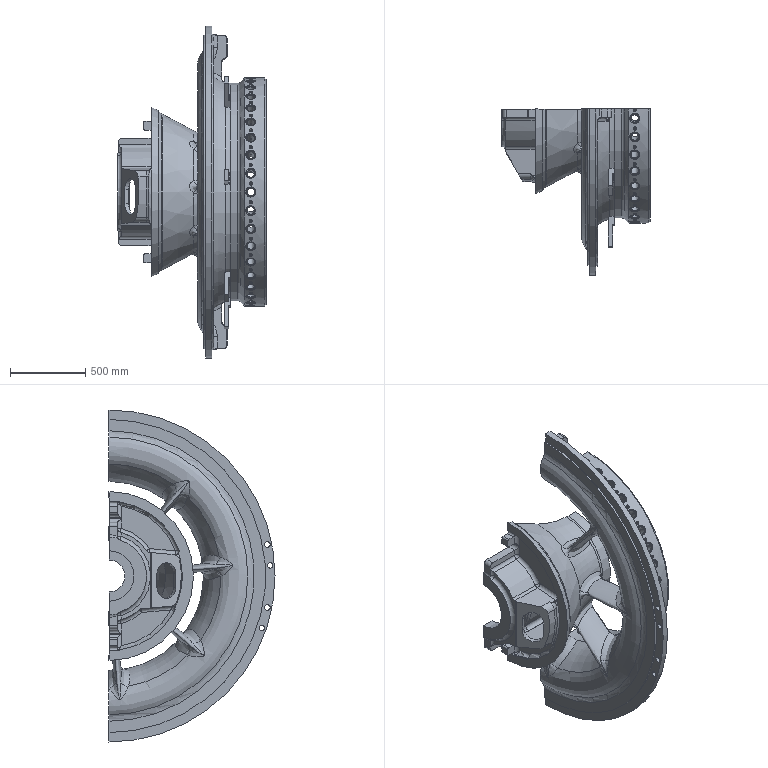Part | SolidWorks | features MBimport 1 | 5 solids | 926 faces | box 985 x 1100 x 2200 mm | volume 275101534 mm3 | cylinder 362 | torus 190 | plane 178 | spline 89 | cone 83 | sphere 24 | commonest cylinder face diameters 50 x83 66.5 x76 20 x46 8 x38 82 x38 6 x12